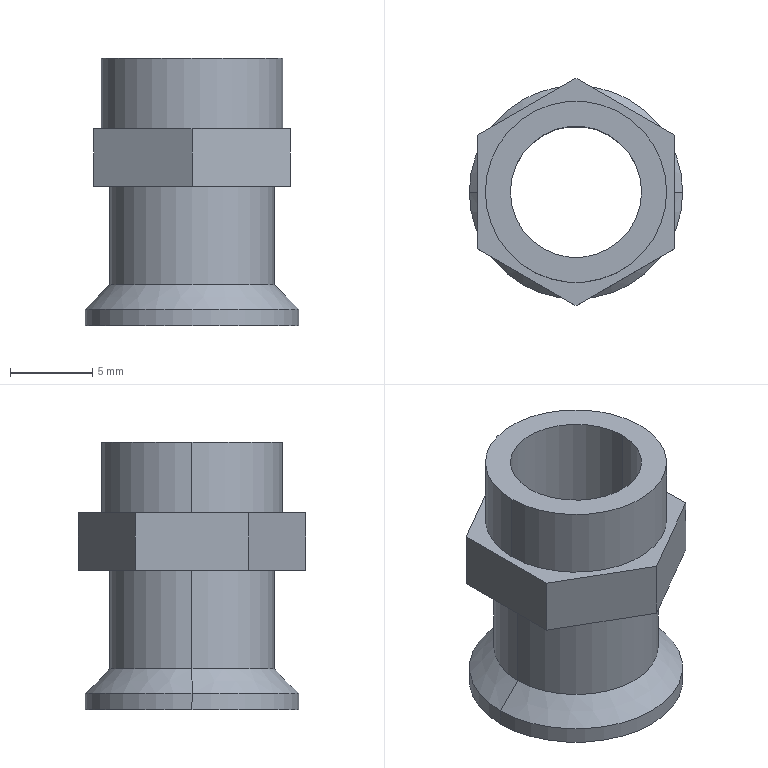Part | STEP file | Sensor nut | 1 solid | 20 faces | box 13 x 13.856 x 16.3 mm | volume 789.56 mm3 | plane 10 | cylinder 8 | cone 2 | commonest cylinder face diameters 8 x2 10 x2 11.042 x2 13 x2
STEP:
#1=CARTESIAN_POINT('',(0.,0.,0.));
#2=DIRECTION('',(0.,0.,1.));
#3=DIRECTION('',(1.,0.,0.));
#4=AXIS2_PLACEMENT_3D('',#1,#2,#3);
#5=CARTESIAN_POINT('',(-4.,0.,7.8));
#6=VERTEX_POINT('',#5);
#7=CARTESIAN_POINT('',(-4.,0.,-8.5));
#8=VERTEX_POINT('',#7);
#9=CARTESIAN_POINT('',(-4.,0.,3.5));
#10=DIRECTION('',(0.,0.,-1.));
#11=VECTOR('',#10,1.);
#12=LINE('',#9,#11);
#13=CARTESIAN_POINT('',(0.,0.,3.5));
#14=DIRECTION('',(0.,0.,-1.));
#15=DIRECTION('',(-1.,0.,0.));
#16=AXIS2_PLACEMENT_3D('',#13,#14,#15);
#17=CYLINDRICAL_SURFACE('',#16,4.);
#18=CARTESIAN_POINT('',(6.283,0.));
#19=DIRECTION('',(0.,1.));
#20=VECTOR('',#19,1.);
#21=LINE('',#18,#20);
#22=(GEOMETRIC_REPRESENTATION_CONTEXT(2)PARAMETRIC_REPRESENTATION_CONTEXT()REPRESENTATION_CONTEXT('',''));
#23=DEFINITIONAL_REPRESENTATION('',(#21),#22);
#24=PCURVE('',#17,#23);
#25=CARTESIAN_POINT('',(0.,0.,3.5));
#26=DIRECTION('',(0.,0.,-1.));
#27=DIRECTION('',(-1.,0.,0.));
#28=AXIS2_PLACEMENT_3D('',#25,#26,#27);
#29=CYLINDRICAL_SURFACE('',#28,4.);
#30=CARTESIAN_POINT('',(0.,0.));
#31=DIRECTION('',(0.,1.));
#32=VECTOR('',#31,1.);
#33=LINE('',#30,#32);
#34=(GEOMETRIC_REPRESENTATION_CONTEXT(2)PARAMETRIC_REPRESENTATION_CONTEXT()REPRESENTATION_CONTEXT('',''));
#35=DEFINITIONAL_REPRESENTATION('',(#33),#34);
#36=PCURVE('',#29,#35);
#37=SURFACE_CURVE('',#12,(#24,#36),.PCURVE_S1.);
#38=EDGE_CURVE('',#6,#8,#37,.T.);
#39=ORIENTED_EDGE('',*,*,#38,.T.);
#40=CARTESIAN_POINT('',(4.,0.,-8.5));
#41=VERTEX_POINT('',#40);
#42=CARTESIAN_POINT('',(0.,0.,-8.5));
#43=DIRECTION('',(0.,0.,1.));
#44=DIRECTION('',(-1.,0.,0.));
#45=AXIS2_PLACEMENT_3D('',#42,#43,#44);
#46=CIRCLE('',#45,4.);
#47=CARTESIAN_POINT('',(6.283,12.));
#48=DIRECTION('',(-1.,0.));
#49=VECTOR('',#48,1.);
#50=LINE('',#47,#49);
#51=(GEOMETRIC_REPRESENTATION_CONTEXT(2)PARAMETRIC_REPRESENTATION_CONTEXT()REPRESENTATION_CONTEXT('',''));
#52=DEFINITIONAL_REPRESENTATION('',(#50),#51);
#53=PCURVE('',#17,#52);
#54=CARTESIAN_POINT('',(6.5,0.,-8.5));
#55=DIRECTION('',(0.,0.,-1.));
#56=DIRECTION('',(-1.,0.,0.));
#57=AXIS2_PLACEMENT_3D('',#54,#55,#56);
#58=PLANE('',#57);
#59=CARTESIAN_POINT('',(10.5,0.));
#60=CARTESIAN_POINT('',(10.5,-6.928));
#61=CARTESIAN_POINT('',(4.5,-3.464));
#62=CARTESIAN_POINT('',(-1.5,0.));
#63=CARTESIAN_POINT('',(4.5,3.464));
#64=CARTESIAN_POINT('',(10.5,6.928));
#65=CARTESIAN_POINT('',(10.5,0.));
#66=(BOUNDED_CURVE()B_SPLINE_CURVE(2,(#59,#60,#61,#62,#63,#64,#65),.UNSPECIFIED.,.T.,.F.)B_SPLINE_CURVE_WITH_KNOTS((1,2,2,2,2,1),(-2.094,0.,2.094,4.189,6.283,8.378),.UNSPECIFIED.)CURVE()GEOMETRIC_REPRESENTATION_ITEM()RATIONAL_B_SPLINE_CURVE((1.,0.5,1.,0.5,1.,0.5,1.))REPRESENTATION_ITEM(''));
#67=(GEOMETRIC_REPRESENTATION_CONTEXT(2)PARAMETRIC_REPRESENTATION_CONTEXT()REPRESENTATION_CONTEXT('',''));
#68=DEFINITIONAL_REPRESENTATION('',(#66),#67);
#69=PCURVE('',#58,#68);
#70=SURFACE_CURVE('',#46,(#53,#69),.PCURVE_S1.);
#71=EDGE_CURVE('',#8,#41,#70,.T.);
#72=ORIENTED_EDGE('',*,*,#71,.T.);
#73=CARTESIAN_POINT('',(4.,0.,7.8));
#74=VERTEX_POINT('',#73);
#75=CARTESIAN_POINT('',(4.,0.,3.5));
#76=DIRECTION('',(0.,0.,-1.));
#77=VECTOR('',#76,1.);
#78=LINE('',#75,#77);
#79=CARTESIAN_POINT('',(3.142,0.));
#80=DIRECTION('',(0.,1.));
#81=VECTOR('',#80,1.);
#82=LINE('',#79,#81);
#83=(GEOMETRIC_REPRESENTATION_CONTEXT(2)PARAMETRIC_REPRESENTATION_CONTEXT()REPRESENTATION_CONTEXT('',''));
#84=DEFINITIONAL_REPRESENTATION('',(#82),#83);
#85=PCURVE('',#17,#84);
#86=CARTESIAN_POINT('',(3.142,0.));
#87=DIRECTION('',(0.,1.));
#88=VECTOR('',#87,1.);
#89=LINE('',#86,#88);
#90=(GEOMETRIC_REPRESENTATION_CONTEXT(2)PARAMETRIC_REPRESENTATION_CONTEXT()REPRESENTATION_CONTEXT('',''));
#91=DEFINITIONAL_REPRESENTATION('',(#89),#90);
#92=PCURVE('',#29,#91);
#93=SURFACE_CURVE('',#78,(#85,#92),.PCURVE_S1.);
#94=EDGE_CURVE('',#74,#41,#93,.T.);
#95=ORIENTED_EDGE('',*,*,#94,.F.);
#96=CARTESIAN_POINT('',(0.,0.,7.8));
#97=DIRECTION('',(0.,0.,-1.));
#98=DIRECTION('',(-1.,0.,0.));
#99=AXIS2_PLACEMENT_3D('',#96,#97,#98);
#100=CIRCLE('',#99,4.);
#101=CARTESIAN_POINT('',(0.,-4.3));
#102=DIRECTION('',(1.,0.));
#103=VECTOR('',#102,1.);
#104=LINE('',#101,#103);
#105=(GEOMETRIC_REPRESENTATION_CONTEXT(2)PARAMETRIC_REPRESENTATION_CONTEXT()REPRESENTATION_CONTEXT('',''));
#106=DEFINITIONAL_REPRESENTATION('',(#104),#105);
#107=PCURVE('',#17,#106);
#108=CARTESIAN_POINT('',(4.,0.,7.8));
#109=DIRECTION('',(0.,0.,1.));
#110=DIRECTION('',(1.,0.,0.));
#111=AXIS2_PLACEMENT_3D('',#108,#109,#110);
#112=PLANE('',#111);
#113=CARTESIAN_POINT('',(-8.,0.));
#114=CARTESIAN_POINT('',(-8.,6.928));
#115=CARTESIAN_POINT('',(-2.,3.464));
#116=CARTESIAN_POINT('',(4.,0.));
#117=CARTESIAN_POINT('',(-2.,-3.464));
#118=CARTESIAN_POINT('',(-8.,-6.928));
#119=CARTESIAN_POINT('',(-8.,0.));
#120=(BOUNDED_CURVE()B_SPLINE_CURVE(2,(#113,#114,#115,#116,#117,#118,#119),.UNSPECIFIED.,.T.,.F.)B_SPLINE_CURVE_WITH_KNOTS((1,2,2,2,2,1),(-2.094,0.,2.094,4.189,6.283,8.378),.UNSPECIFIED.)CURVE()GEOMETRIC_REPRESENTATION_ITEM()RATIONAL_B_SPLINE_CURVE((1.,0.5,1.,0.5,1.,0.5,1.))REPRESENTATION_ITEM(''));
#121=(GEOMETRIC_REPRESENTATION_CONTEXT(2)PARAMETRIC_REPRESENTATION_CONTEXT()REPRESENTATION_CONTEXT('',''));
#122=DEFINITIONAL_REPRESENTATION('',(#120),#121);
#123=PCURVE('',#112,#122);
#124=SURFACE_CURVE('',#100,(#107,#123),.PCURVE_S1.);
#125=EDGE_CURVE('',#74,#6,#124,.T.);
#126=ORIENTED_EDGE('',*,*,#125,.T.);
#127=EDGE_LOOP('',(#39,#72,#95,#126));
#128=FACE_BOUND('',#127,.F.);
#129=ADVANCED_FACE('',(#128),#17,.F.);
#130=CARTESIAN_POINT('',(5.521,0.,3.5));
#131=VERTEX_POINT('',#130);
#132=CARTESIAN_POINT('',(-5.521,0.,3.5));
#133=VERTEX_POINT('',#132);
#134=CARTESIAN_POINT('',(0.,0.,3.5));
#135=DIRECTION('',(0.,0.,1.));
#136=DIRECTION('',(1.,0.,0.));
#137=AXIS2_PLACEMENT_3D('',#134,#135,#136);
#138=CIRCLE('',#137,5.521);
#139=CARTESIAN_POINT('',(0.,0.,0.));
#140=DIRECTION('',(0.,0.,1.));
#141=DIRECTION('',(1.,0.,0.));
#142=AXIS2_PLACEMENT_3D('',#139,#140,#141);
#143=CYLINDRICAL_SURFACE('',#142,5.521);
#144=CARTESIAN_POINT('',(0.,3.5));
#145=DIRECTION('',(1.,0.));
#146=VECTOR('',#145,1.);
#147=LINE('',#144,#146);
#148=(GEOMETRIC_REPRESENTATION_CONTEXT(2)PARAMETRIC_REPRESENTATION_CONTEXT()REPRESENTATION_CONTEXT('',''));
#149=DEFINITIONAL_REPRESENTATION('',(#147),#148);
#150=PCURVE('',#143,#149);
#151=CARTESIAN_POINT('',(0.,6.928,3.5));
#152=DIRECTION('',(0.,0.,1.));
#153=DIRECTION('',(1.,0.,0.));
#154=AXIS2_PLACEMENT_3D('',#151,#152,#153);
#155=PLANE('',#154);
#156=CARTESIAN_POINT('',(0.,-6.928));
#157=DIRECTION('',(1.,0.));
#158=AXIS2_PLACEMENT_2D('',#156,#157);
#159=CIRCLE('',#158,5.521);
#160=(GEOMETRIC_REPRESENTATION_CONTEXT(2)PARAMETRIC_REPRESENTATION_CONTEXT()REPRESENTATION_CONTEXT('',''));
#161=DEFINITIONAL_REPRESENTATION('',(#159),#160);
#162=PCURVE('',#155,#161);
#163=SURFACE_CURVE('',#138,(#150,#162),.PCURVE_S1.);
#164=EDGE_CURVE('',#131,#133,#163,.T.);
#165=ORIENTED_EDGE('',*,*,#164,.T.);
#166=CARTESIAN_POINT('',(-5.521,0.,7.8));
#167=VERTEX_POINT('',#166);
#168=CARTESIAN_POINT('',(-5.521,0.,0.));
#169=DIRECTION('',(0.,0.,1.));
#170=VECTOR('',#169,1.);
#171=LINE('',#168,#170);
#172=CARTESIAN_POINT('',(3.142,0.));
#173=DIRECTION('',(0.,1.));
#174=VECTOR('',#173,1.);
#175=LINE('',#172,#174);
#176=(GEOMETRIC_REPRESENTATION_CONTEXT(2)PARAMETRIC_REPRESENTATION_CONTEXT()REPRESENTATION_CONTEXT('',''));
#177=DEFINITIONAL_REPRESENTATION('',(#175),#176);
#178=PCURVE('',#143,#177);
#179=CARTESIAN_POINT('',(0.,0.,0.));
#180=DIRECTION('',(0.,0.,1.));
#181=DIRECTION('',(1.,0.,0.));
#182=AXIS2_PLACEMENT_3D('',#179,#180,#181);
#183=CYLINDRICAL_SURFACE('',#182,5.521);
#184=CARTESIAN_POINT('',(3.142,0.));
#185=DIRECTION('',(0.,1.));
#186=VECTOR('',#185,1.);
#187=LINE('',#184,#186);
#188=(GEOMETRIC_REPRESENTATION_CONTEXT(2)PARAMETRIC_REPRESENTATION_CONTEXT()REPRESENTATION_CONTEXT('',''));
#189=DEFINITIONAL_REPRESENTATION('',(#187),#188);
#190=PCURVE('',#183,#189);
#191=SURFACE_CURVE('',#171,(#178,#190),.PCURVE_S1.);
#192=EDGE_CURVE('',#133,#167,#191,.T.);
#193=ORIENTED_EDGE('',*,*,#192,.T.);
#194=CARTESIAN_POINT('',(5.521,0.,7.8));
#195=VERTEX_POINT('',#194);
#196=CARTESIAN_POINT('',(0.,0.,7.8));
#197=DIRECTION('',(0.,0.,1.));
#198=DIRECTION('',(1.,0.,0.));
#199=AXIS2_PLACEMENT_3D('',#196,#197,#198);
#200=CIRCLE('',#199,5.521);
#201=CARTESIAN_POINT('',(0.,7.8));
#202=DIRECTION('',(1.,0.));
#203=VECTOR('',#202,1.);
#204=LINE('',#201,#203);
#205=(GEOMETRIC_REPRESENTATION_CONTEXT(2)PARAMETRIC_REPRESENTATION_CONTEXT()REPRESENTATION_CONTEXT('',''));
#206=DEFINITIONAL_REPRESENTATION('',(#204),#205);
#207=PCURVE('',#143,#206);
#208=CARTESIAN_POINT('',(-4.,0.));
#209=DIRECTION('',(1.,0.));
#210=AXIS2_PLACEMENT_2D('',#208,#209);
#211=CIRCLE('',#210,5.521);
#212=(GEOMETRIC_REPRESENTATION_CONTEXT(2)PARAMETRIC_REPRESENTATION_CONTEXT()REPRESENTATION_CONTEXT('',''));
#213=DEFINITIONAL_REPRESENTATION('',(#211),#212);
#214=PCURVE('',#112,#213);
#215=SURFACE_CURVE('',#200,(#207,#214),.PCURVE_S1.);
#216=EDGE_CURVE('',#195,#167,#215,.T.);
#217=ORIENTED_EDGE('',*,*,#216,.F.);
#218=CARTESIAN_POINT('',(5.521,0.,0.));
#219=DIRECTION('',(0.,0.,1.));
#220=VECTOR('',#219,1.);
#221=LINE('',#218,#220);
#222=CARTESIAN_POINT('',(0.,0.));
#223=DIRECTION('',(0.,1.));
#224=VECTOR('',#223,1.);
#225=LINE('',#222,#224);
#226=(GEOMETRIC_REPRESENTATION_CONTEXT(2)PARAMETRIC_REPRESENTATION_CONTEXT()REPRESENTATION_CONTEXT('',''));
#227=DEFINITIONAL_REPRESENTATION('',(#225),#226);
#228=PCURVE('',#143,#227);
#229=CARTESIAN_POINT('',(6.283,0.));
#230=DIRECTION('',(0.,1.));
#231=VECTOR('',#230,1.);
#232=LINE('',#229,#231);
#233=(GEOMETRIC_REPRESENTATION_CONTEXT(2)PARAMETRIC_REPRESENTATION_CONTEXT()REPRESENTATION_CONTEXT('',''));
#234=DEFINITIONAL_REPRESENTATION('',(#232),#233);
#235=PCURVE('',#183,#234);
#236=SURFACE_CURVE('',#221,(#228,#235),.PCURVE_S1.);
#237=EDGE_CURVE('',#131,#195,#236,.T.);
#238=ORIENTED_EDGE('',*,*,#237,.F.);
#239=EDGE_LOOP('',(#165,#193,#217,#238));
#240=FACE_BOUND('',#239,.T.);
#241=ADVANCED_FACE('',(#240),#143,.T.);
#242=CARTESIAN_POINT('',(-6.5,0.,-8.5));
#243=VERTEX_POINT('',#242);
#244=CARTESIAN_POINT('',(6.5,0.,-8.5));
#245=VERTEX_POINT('',#244);
#246=CARTESIAN_POINT('',(0.,0.,-8.5));
#247=DIRECTION('',(0.,0.,-1.));
#248=DIRECTION('',(1.,0.,0.));
#249=AXIS2_PLACEMENT_3D('',#246,#247,#248);
#250=CIRCLE('',#249,6.5);
#251=CARTESIAN_POINT('',(0.,0.,0.));
#252=DIRECTION('',(0.,0.,1.));
#253=DIRECTION('',(1.,0.,0.));
#254=AXIS2_PLACEMENT_3D('',#251,#252,#253);
#255=CYLINDRICAL_SURFACE('',#254,6.5);
#256=CARTESIAN_POINT('',(6.283,-8.5));
#257=DIRECTION('',(-1.,0.));
#258=VECTOR('',#257,1.);
#259=LINE('',#256,#258);
#260=(GEOMETRIC_REPRESENTATION_CONTEXT(2)PARAMETRIC_REPRESENTATION_CONTEXT()REPRESENTATION_CONTEXT('',''));
#261=DEFINITIONAL_REPRESENTATION('',(#259),#260);
#262=PCURVE('',#255,#261);
#263=CARTESIAN_POINT('',(6.5,0.));
#264=DIRECTION('',(-1.,0.));
#265=AXIS2_PLACEMENT_2D('',#263,#264);
#266=CIRCLE('',#265,6.5);
#267=(GEOMETRIC_REPRESENTATION_CONTEXT(2)PARAMETRIC_REPRESENTATION_CONTEXT()REPRESENTATION_CONTEXT('',''));
#268=DEFINITIONAL_REPRESENTATION('',(#266),#267);
#269=PCURVE('',#58,#268);
#270=SURFACE_CURVE('',#250,(#262,#269),.PCURVE_S1.);
#271=EDGE_CURVE('',#243,#245,#270,.T.);
#272=ORIENTED_EDGE('',*,*,#271,.F.);
#273=CARTESIAN_POINT('',(-6.5,0.,-7.5));
#274=VERTEX_POINT('',#273);
#275=CARTESIAN_POINT('',(-6.5,0.,0.));
#276=DIRECTION('',(0.,0.,1.));
#277=VECTOR('',#276,1.);
#278=LINE('',#275,#277);
#279=CARTESIAN_POINT('',(3.142,0.));
#280=DIRECTION('',(0.,1.));
#281=VECTOR('',#280,1.);
#282=LINE('',#279,#281);
#283=(GEOMETRIC_REPRESENTATION_CONTEXT(2)PARAMETRIC_REPRESENTATION_CONTEXT()REPRESENTATION_CONTEXT('',''));
#284=DEFINITIONAL_REPRESENTATION('',(#282),#283);
#285=PCURVE('',#255,#284);
#286=CARTESIAN_POINT('',(0.,0.,0.));
#287=DIRECTION('',(0.,0.,1.));
#288=DIRECTION('',(1.,0.,0.));
#289=AXIS2_PLACEMENT_3D('',#286,#287,#288);
#290=CYLINDRICAL_SURFACE('',#289,6.5);
#291=CARTESIAN_POINT('',(3.142,0.));
#292=DIRECTION('',(0.,1.));
#293=VECTOR('',#292,1.);
#294=LINE('',#291,#293);
#295=(GEOMETRIC_REPRESENTATION_CONTEXT(2)PARAMETRIC_REPRESENTATION_CONTEXT()REPRESENTATION_CONTEXT('',''));
#296=DEFINITIONAL_REPRESENTATION('',(#294),#295);
#297=PCURVE('',#290,#296);
#298=SURFACE_CURVE('',#278,(#285,#297),.PCURVE_S1.);
#299=EDGE_CURVE('',#243,#274,#298,.T.);
#300=ORIENTED_EDGE('',*,*,#299,.T.);
#301=CARTESIAN_POINT('',(6.5,0.,-7.5));
#302=VERTEX_POINT('',#301);
#303=CARTESIAN_POINT('',(0.,0.,-7.5));
#304=DIRECTION('',(0.,0.,-1.));
#305=DIRECTION('',(1.,0.,0.));
#306=AXIS2_PLACEMENT_3D('',#303,#304,#305);
#307=CIRCLE('',#306,6.5);
#308=CARTESIAN_POINT('',(6.283,-7.5));
#309=DIRECTION('',(-1.,0.));
#310=VECTOR('',#309,1.);
#311=LINE('',#308,#310);
#312=(GEOMETRIC_REPRESENTATION_CONTEXT(2)PARAMETRIC_REPRESENTATION_CONTEXT()REPRESENTATION_CONTEXT('',''));
#313=DEFINITIONAL_REPRESENTATION('',(#311),#312);
#314=PCURVE('',#255,#313);
#315=CARTESIAN_POINT('',(0.,0.,-7.5));
#316=DIRECTION('',(0.,0.,-1.));
#317=DIRECTION('',(-1.,0.,0.));
#318=AXIS2_PLACEMENT_3D('',#315,#316,#317);
#319=CONICAL_SURFACE('',#318,6.5,0.7854);
#320=CARTESIAN_POINT('',(-3.142,0.));
#321=DIRECTION('',(1.,0.));
#322=VECTOR('',#321,1.);
#323=LINE('',#320,#322);
#324=(GEOMETRIC_REPRESENTATION_CONTEXT(2)PARAMETRIC_REPRESENTATION_CONTEXT()REPRESENTATION_CONTEXT('',''));
#325=DEFINITIONAL_REPRESENTATION('',(#323),#324);
#326=PCURVE('',#319,#325);
#327=SURFACE_CURVE('',#307,(#314,#326),.PCURVE_S1.);
#328=EDGE_CURVE('',#274,#302,#327,.T.);
#329=ORIENTED_EDGE('',*,*,#328,.T.);
#330=CARTESIAN_POINT('',(6.5,0.,0.));
#331=DIRECTION('',(0.,0.,1.));
#332=VECTOR('',#331,1.);
#333=LINE('',#330,#332);
#334=CARTESIAN_POINT('',(0.,0.));
#335=DIRECTION('',(0.,1.));
#336=VECTOR('',#335,1.);
#337=LINE('',#334,#336);
#338=(GEOMETRIC_REPRESENTATION_CONTEXT(2)PARAMETRIC_REPRESENTATION_CONTEXT()REPRESENTATION_CONTEXT('',''));
#339=DEFINITIONAL_REPRESENTATION('',(#337),#338);
#340=PCURVE('',#255,#339);
#341=CARTESIAN_POINT('',(6.283,0.));
#342=DIRECTION('',(0.,1.));
#343=VECTOR('',#342,1.);
#344=LINE('',#341,#343);
#345=(GEOMETRIC_REPRESENTATION_CONTEXT(2)PARAMETRIC_REPRESENTATION_CONTEXT()REPRESENTATION_CONTEXT('',''));
#346=DEFINITIONAL_REPRESENTATION('',(#344),#345);
#347=PCURVE('',#290,#346);
#348=SURFACE_CURVE('',#333,(#340,#347),.PCURVE_S1.);
#349=EDGE_CURVE('',#245,#302,#348,.T.);
#350=ORIENTED_EDGE('',*,*,#349,.F.);
#351=EDGE_LOOP('',(#272,#300,#329,#350));
#352=FACE_BOUND('',#351,.T.);
#353=ADVANCED_FACE('',(#352),#255,.T.);
#354=CARTESIAN_POINT('',(-5.,0.,-6.));
#355=VERTEX_POINT('',#354);
#356=CARTESIAN_POINT('',(5.,0.,-6.));
#357=VERTEX_POINT('',#356);
#358=CARTESIAN_POINT('',(0.,0.,-6.));
#359=DIRECTION('',(0.,0.,-1.));
#360=DIRECTION('',(-1.,0.,0.));
#361=AXIS2_PLACEMENT_3D('',#358,#359,#360);
#362=CIRCLE('',#361,5.);
#363=CARTESIAN_POINT('',(0.,-1.5));
#364=DIRECTION('',(1.,0.));
#365=VECTOR('',#364,1.);
#366=LINE('',#363,#365);
#367=(GEOMETRIC_REPRESENTATION_CONTEXT(2)PARAMETRIC_REPRESENTATION_CONTEXT()REPRESENTATION_CONTEXT('',''));
#368=DEFINITIONAL_REPRESENTATION('',(#366),#367);
#369=PCURVE('',#319,#368);
#370=CARTESIAN_POINT('',(0.,0.,0.));
#371=DIRECTION('',(0.,0.,1.));
#372=DIRECTION('',(1.,0.,0.));
#373=AXIS2_PLACEMENT_3D('',#370,#371,#372);
#374=CYLINDRICAL_SURFACE('',#373,5.);
#375=CARTESIAN_POINT('',(3.142,-6.));
#376=DIRECTION('',(-1.,0.));
#377=VECTOR('',#376,1.);
#378=LINE('',#375,#377);
#379=(GEOMETRIC_REPRESENTATION_CONTEXT(2)PARAMETRIC_REPRESENTATION_CONTEXT()REPRESENTATION_CONTEXT('',''));
#380=DEFINITIONAL_REPRESENTATION('',(#378),#379);
#381=PCURVE('',#374,#380);
#382=SURFACE_CURVE('',#362,(#369,#381),.PCURVE_S1.);
#383=EDGE_CURVE('',#355,#357,#382,.T.);
#384=ORIENTED_EDGE('',*,*,#383,.T.);
#385=CARTESIAN_POINT('',(6.5,0.,-7.5));
#386=DIRECTION('',(0.7071,0.,-0.7071));
#387=VECTOR('',#386,1.);
#388=LINE('',#385,#387);
#389=CARTESIAN_POINT('',(3.142,0.));
#390=DIRECTION('',(0.,1.));
#391=VECTOR('',#390,1.);
#392=LINE('',#389,#391);
#393=(GEOMETRIC_REPRESENTATION_CONTEXT(2)PARAMETRIC_REPRESENTATION_CONTEXT()REPRESENTATION_CONTEXT('',''));
#394=DEFINITIONAL_REPRESENTATION('',(#392),#393);
#395=PCURVE('',#319,#394);
#396=CARTESIAN_POINT('',(0.,0.,-7.5));
#397=DIRECTION('',(0.,0.,-1.));
#398=DIRECTION('',(-1.,0.,0.));
#399=AXIS2_PLACEMENT_3D('',#396,#397,#398);
#400=CONICAL_SURFACE('',#399,6.5,0.7854);
#401=CARTESIAN_POINT('',(3.142,0.));
#402=DIRECTION('',(0.,1.));
#403=VECTOR('',#402,1.);
#404=LINE('',#401,#403);
#405=(GEOMETRIC_REPRESENTATION_CONTEXT(2)PARAMETRIC_REPRESENTATION_CONTEXT()REPRESENTATION_CONTEXT('',''));
#406=DEFINITIONAL_REPRESENTATION('',(#404),#405);
#407=PCURVE('',#400,#406);
#408=SURFACE_CURVE('',#388,(#395,#407),.PCURVE_S1.);
#409=EDGE_CURVE('',#357,#302,#408,.T.);
#410=ORIENTED_EDGE('',*,*,#409,.T.);
#411=ORIENTED_EDGE('',*,*,#328,.F.);
#412=CARTESIAN_POINT('',(-6.5,0.,-7.5));
#413=DIRECTION('',(-0.7071,0.,-0.7071));
#414=VECTOR('',#413,1.);
#415=LINE('',#412,#414);
#416=CARTESIAN_POINT('',(0.,0.));
#417=DIRECTION('',(0.,1.));
#418=VECTOR('',#417,1.);
#419=LINE('',#416,#418);
#420=(GEOMETRIC_REPRESENTATION_CONTEXT(2)PARAMETRIC_REPRESENTATION_CONTEXT()REPRESENTATION_CONTEXT('',''));
#421=DEFINITIONAL_REPRESENTATION('',(#419),#420);
#422=PCURVE('',#319,#421);
#423=CARTESIAN_POINT('',(6.283,0.));
#424=DIRECTION('',(0.,1.));
#425=VECTOR('',#424,1.);
#426=LINE('',#423,#425);
#427=(GEOMETRIC_REPRESENTATION_CONTEXT(2)PARAMETRIC_REPRESENTATION_CONTEXT()REPRESENTATION_CONTEXT('',''));
#428=DEFINITIONAL_REPRESENTATION('',(#426),#427);
#429=PCURVE('',#400,#428);
#430=SURFACE_CURVE('',#415,(#422,#429),.PCURVE_S1.);
#431=EDGE_CURVE('',#355,#274,#430,.T.);
#432=ORIENTED_EDGE('',*,*,#431,.F.);
#433=EDGE_LOOP('',(#384,#410,#411,#432));
#434=FACE_BOUND('',#433,.T.);
#435=ADVANCED_FACE('',(#434),#319,.T.);
#436=ORIENTED_EDGE('',*,*,#383,.F.);
#437=CARTESIAN_POINT('',(-5.,0.,0.));
#438=VERTEX_POINT('',#437);
#439=CARTESIAN_POINT('',(-5.,0.,0.));
#440=DIRECTION('',(0.,0.,1.));
#441=VECTOR('',#440,1.);
#442=LINE('',#439,#441);
#443=CARTESIAN_POINT('',(3.142,0.));
#444=DIRECTION('',(0.,1.));
#445=VECTOR('',#444,1.);
#446=LINE('',#443,#445);
#447=(GEOMETRIC_REPRESENTATION_CONTEXT(2)PARAMETRIC_REPRESENTATION_CONTEXT()REPRESENTATION_CONTEXT('',''));
#448=DEFINITIONAL_REPRESENTATION('',(#446),#447);
#449=PCURVE('',#374,#448);
#450=CARTESIAN_POINT('',(0.,0.,0.));
#451=DIRECTION('',(0.,0.,1.));
#452=DIRECTION('',(1.,0.,0.));
#453=AXIS2_PLACEMENT_3D('',#450,#451,#452);
#454=CYLINDRICAL_SURFACE('',#453,5.);
#455=CARTESIAN_POINT('',(3.142,0.));
#456=DIRECTION('',(0.,1.));
#457=VECTOR('',#456,1.);
#458=LINE('',#455,#457);
#459=(GEOMETRIC_REPRESENTATION_CONTEXT(2)PARAMETRIC_REPRESENTATION_CONTEXT()REPRESENTATION_CONTEXT('',''));
#460=DEFINITIONAL_REPRESENTATION('',(#458),#459);
#461=PCURVE('',#454,#460);
#462=SURFACE_CURVE('',#442,(#449,#461),.PCURVE_S1.);
#463=EDGE_CURVE('',#355,#438,#462,.T.);
#464=ORIENTED_EDGE('',*,*,#463,.T.);
#465=CARTESIAN_POINT('',(5.,0.,0.));
#466=VERTEX_POINT('',#465);
#467=CARTESIAN_POINT('',(0.,0.,0.));
#468=DIRECTION('',(0.,0.,-1.));
#469=DIRECTION('',(1.,0.,0.));
#470=AXIS2_PLACEMENT_3D('',#467,#468,#469);
#471=CIRCLE('',#470,5.);
#472=CARTESIAN_POINT('',(6.283,0.));
#473=DIRECTION('',(-1.,0.));
#474=VECTOR('',#473,1.);
#475=LINE('',#472,#474);
#476=(GEOMETRIC_REPRESENTATION_CONTEXT(2)PARAMETRIC_REPRESENTATION_CONTEXT()REPRESENTATION_CONTEXT('',''));
#477=DEFINITIONAL_REPRESENTATION('',(#475),#476);
#478=PCURVE('',#374,#477);
#479=CARTESIAN_POINT('',(0.,6.928,0.));
#480=DIRECTION('',(0.,0.,1.));
#481=DIRECTION('',(1.,0.,0.));
#482=AXIS2_PLACEMENT_3D('',#479,#480,#481);
#483=PLANE('',#482);
#484=CARTESIAN_POINT('',(5.,-6.928));
#485=CARTESIAN_POINT('',(5.,-15.588));
#486=CARTESIAN_POINT('',(-2.5,-11.258));
#487=CARTESIAN_POINT('',(-10.,-6.928));
#488=CARTESIAN_POINT('',(-2.5,-2.598));
#489=CARTESIAN_POINT('',(5.,1.732));
#490=CARTESIAN_POINT('',(5.,-6.928));
#491=(BOUNDED_CURVE()B_SPLINE_CURVE(2,(#484,#485,#486,#487,#488,#489,#490),.UNSPECIFIED.,.T.,.F.)B_SPLINE_CURVE_WITH_KNOTS((1,2,2,2,2,1),(-2.094,0.,2.094,4.189,6.283,8.378),.UNSPECIFIED.)CURVE()GEOMETRIC_REPRESENTATION_ITEM()RATIONAL_B_SPLINE_CURVE((1.,0.5,1.,0.5,1.,0.5,1.))REPRESENTATION_ITEM(''));
#492=(GEOMETRIC_REPRESENTATION_CONTEXT(2)PARAMETRIC_REPRESENTATION_CONTEXT()REPRESENTATION_CONTEXT('',''));
#493=DEFINITIONAL_REPRESENTATION('',(#491),#492);
#494=PCURVE('',#483,#493);
#495=SURFACE_CURVE('',#471,(#478,#494),.PCURVE_S1.);
#496=EDGE_CURVE('',#438,#466,#495,.T.);
#497=ORIENTED_EDGE('',*,*,#496,.T.);
#498=CARTESIAN_POINT('',(5.,0.,0.));
#499=DIRECTION('',(0.,0.,1.));
#500=VECTOR('',#499,1.);
#501=LINE('',#498,#500);
#502=CARTESIAN_POINT('',(0.,0.));
#503=DIRECTION('',(0.,1.));
#504=VECTOR('',#503,1.);
#505=LINE('',#502,#504);
#506=(GEOMETRIC_REPRESENTATION_CONTEXT(2)PARAMETRIC_REPRESENTATION_CONTEXT()REPRESENTATION_CONTEXT('',''));
#507=DEFINITIONAL_REPRESENTATION('',(#505),#506);
#508=PCURVE('',#374,#507);
#509=CARTESIAN_POINT('',(6.283,0.));
#510=DIRECTION('',(0.,1.));
#511=VECTOR('',#510,1.);
#512=LINE('',#509,#511);
#513=(GEOMETRIC_REPRESENTATION_CONTEXT(2)PARAMETRIC_REPRESENTATION_CONTEXT()REPRESENTATION_CONTEXT('',''));
#514=DEFINITIONAL_REPRESENTATION('',(#512),#513);
#515=PCURVE('',#454,#514);
#516=SURFACE_CURVE('',#501,(#508,#515),.PCURVE_S1.);
#517=EDGE_CURVE('',#357,#466,#516,.T.);
#518=ORIENTED_EDGE('',*,*,#517,.F.);
#519=EDGE_LOOP('',(#436,#464,#497,#518));
#520=FACE_BOUND('',#519,.T.);
#521=ADVANCED_FACE('',(#520),#374,.T.);
#522=CARTESIAN_POINT('',(0.,0.,-8.5));
#523=DIRECTION('',(0.,0.,1.));
#524=DIRECTION('',(-1.,0.,0.));
#525=AXIS2_PLACEMENT_3D('',#522,#523,#524);
#526=CIRCLE('',#525,4.);
#527=CARTESIAN_POINT('',(6.283,12.));
#528=DIRECTION('',(-1.,0.));
#529=VECTOR('',#528,1.);
#530=LINE('',#527,#529);
#531=(GEOMETRIC_REPRESENTATION_CONTEXT(2)PARAMETRIC_REPRESENTATION_CONTEXT()REPRESENTATION_CONTEXT('',''));
#532=DEFINITIONAL_REPRESENTATION('',(#530),#531);
#533=PCURVE('',#29,#532);
#534=CARTESIAN_POINT('',(10.5,0.));
#535=CARTESIAN_POINT('',(10.5,-6.928));
#536=CARTESIAN_POINT('',(4.5,-3.464));
#537=CARTESIAN_POINT('',(-1.5,0.));
#538=CARTESIAN_POINT('',(4.5,3.464));
#539=CARTESIAN_POINT('',(10.5,6.928));
#540=CARTESIAN_POINT('',(10.5,0.));
#541=(BOUNDED_CURVE()B_SPLINE_CURVE(2,(#534,#535,#536,#537,#538,#539,#540),.UNSPECIFIED.,.T.,.F.)B_SPLINE_CURVE_WITH_KNOTS((1,2,2,2,2,1),(-2.094,0.,2.094,4.189,6.283,8.378),.UNSPECIFIED.)CURVE()GEOMETRIC_REPRESENTATION_ITEM()RATIONAL_B_SPLINE_CURVE((1.,0.5,1.,0.5,1.,0.5,1.))REPRESENTATION_ITEM(''));
#542=(GEOMETRIC_REPRESENTATION_CONTEXT(2)PARAMETRIC_REPRESENTATION_CONTEXT()REPRESENTATION_CONTEXT('',''));
#543=DEFINITIONAL_REPRESENTATION('',(#541),#542);
#544=PCURVE('',#58,#543);
#545=SURFACE_CURVE('',#526,(#533,#544),.PCURVE_S1.);
#546=EDGE_CURVE('',#41,#8,#545,.T.);
#547=ORIENTED_EDGE('',*,*,#546,.T.);
#548=ORIENTED_EDGE('',*,*,#38,.F.);
#549=CARTESIAN_POINT('',(0.,0.,7.8));
#550=DIRECTION('',(0.,0.,-1.));
#551=DIRECTION('',(-1.,0.,0.));
#552=AXIS2_PLACEMENT_3D('',#549,#550,#551);
#553=CIRCLE('',#552,4.);
#554=CARTESIAN_POINT('',(0.,-4.3));
#555=DIRECTION('',(1.,0.));
#556=VECTOR('',#555,1.);
#557=LINE('',#554,#556);
#558=(GEOMETRIC_REPRESENTATION_CONTEXT(2)PARAMETRIC_REPRESENTATION_CONTEXT()REPRESENTATION_CONTEXT('',''));
#559=DEFINITIONAL_REPRESENTATION('',(#557),#558);
#560=PCURVE('',#29,#559);
#561=CARTESIAN_POINT('',(-8.,0.));
#562=CARTESIAN_POINT('',(-8.,6.928));
#563=CARTESIAN_POINT('',(-2.,3.464));
#564=CARTESIAN_POINT('',(4.,0.));
#565=CARTESIAN_POINT('',(-2.,-3.464));
#566=CARTESIAN_POINT('',(-8.,-6.928));
#567=CARTESIAN_POINT('',(-8.,0.));
#568=(BOUNDED_CURVE()B_SPLINE_CURVE(2,(#561,#562,#563,#564,#565,#566,#567),.UNSPECIFIED.,.T.,.F.)B_SPLINE_CURVE_WITH_KNOTS((1,2,2,2,2,1),(-2.094,0.,2.094,4.189,6.283,8.378),.UNSPECIFIED.)CURVE()GEOMETRIC_REPRESENTATION_ITEM()RATIONAL_B_SPLINE_CURVE((1.,0.5,1.,0.5,1.,0.5,1.))REPRESENTATION_ITEM(''));
#569=(GEOMETRIC_REPRESENTATION_CONTEXT(2)PARAMETRIC_REPRESENTATION_CONTEXT()REPRESENTATION_CONTEXT('',''));
#570=DEFINITIONAL_REPRESENTATION('',(#568),#569);
#571=PCURVE('',#112,#570);
#572=SURFACE_CURVE('',#553,(#560,#571),.PCURVE_S1.);
#573=EDGE_CURVE('',#6,#74,#572,.T.);
#574=ORIENTED_EDGE('',*,*,#573,.T.);
#575=ORIENTED_EDGE('',*,*,#94,.T.);
#576=EDGE_LOOP('',(#547,#548,#574,#575));
#577=FACE_BOUND('',#576,.F.);
#578=ADVANCED_FACE('',(#577),#29,.F.);
#579=ORIENTED_EDGE('',*,*,#573,.T.);
#580=ORIENTED_EDGE('',*,*,#125,.T.);
#581=EDGE_LOOP('',(#579,#580));
#582=FACE_BOUND('',#581,.T.);
#583=ORIENTED_EDGE('',*,*,#216,.T.);
#584=CARTESIAN_POINT('',(0.,0.,7.8));
#585=DIRECTION('',(0.,0.,1.));
#586=DIRECTION('',(1.,0.,0.));
#587=AXIS2_PLACEMENT_3D('',#584,#585,#586);
#588=CIRCLE('',#587,5.521);
#589=CARTESIAN_POINT('',(-4.,0.));
#590=DIRECTION('',(1.,0.));
#591=AXIS2_PLACEMENT_2D('',#589,#590);
#592=CIRCLE('',#591,5.521);
#593=(GEOMETRIC_REPRESENTATION_CONTEXT(2)PARAMETRIC_REPRESENTATION_CONTEXT()REPRESENTATION_CONTEXT('',''));
#594=DEFINITIONAL_REPRESENTATION('',(#592),#593);
#595=PCURVE('',#112,#594);
#596=CARTESIAN_POINT('',(0.,7.8));
#597=DIRECTION('',(1.,0.));
#598=VECTOR('',#597,1.);
#599=LINE('',#596,#598);
#600=(GEOMETRIC_REPRESENTATION_CONTEXT(2)PARAMETRIC_REPRESENTATION_CONTEXT()REPRESENTATION_CONTEXT('',''));
#601=DEFINITIONAL_REPRESENTATION('',(#599),#600);
#602=PCURVE('',#183,#601);
#603=SURFACE_CURVE('',#588,(#595,#602),.PCURVE_S1.);
#604=EDGE_CURVE('',#167,#195,#603,.T.);
#605=ORIENTED_EDGE('',*,*,#604,.T.);
#606=EDGE_LOOP('',(#583,#605));
#607=FACE_BOUND('',#606,.T.);
#608=ADVANCED_FACE('',(#582,#607),#112,.T.);
#609=CARTESIAN_POINT('',(0.,0.,-8.5));
#610=DIRECTION('',(0.,0.,-1.));
#611=DIRECTION('',(1.,0.,0.));
#612=AXIS2_PLACEMENT_3D('',#609,#610,#611);
#613=CIRCLE('',#612,6.5);
#614=CARTESIAN_POINT('',(6.5,0.));
#615=DIRECTION('',(-1.,0.));
#616=AXIS2_PLACEMENT_2D('',#614,#615);
#617=CIRCLE('',#616,6.5);
#618=(GEOMETRIC_REPRESENTATION_CONTEXT(2)PARAMETRIC_REPRESENTATION_CONTEXT()REPRESENTATION_CONTEXT('',''));
#619=DEFINITIONAL_REPRESENTATION('',(#617),#618);
#620=PCURVE('',#58,#619);
#621=CARTESIAN_POINT('',(6.283,-8.5));
#622=DIRECTION('',(-1.,0.));
#623=VECTOR('',#622,1.);
#624=LINE('',#621,#623);
#625=(GEOMETRIC_REPRESENTATION_CONTEXT(2)PARAMETRIC_REPRESENTATION_CONTEXT()REPRESENTATION_CONTEXT('',''));
#626=DEFINITIONAL_REPRESENTATION('',(#624),#625);
#627=PCURVE('',#290,#626);
#628=SURFACE_CURVE('',#613,(#620,#627),.PCURVE_S1.);
#629=EDGE_CURVE('',#245,#243,#628,.T.);
#630=ORIENTED_EDGE('',*,*,#629,.T.);
#631=ORIENTED_EDGE('',*,*,#271,.T.);
#632=EDGE_LOOP('',(#630,#631));
#633=FACE_BOUND('',#632,.T.);
#634=ORIENTED_EDGE('',*,*,#71,.T.);
#635=ORIENTED_EDGE('',*,*,#546,.T.);
#636=EDGE_LOOP('',(#634,#635));
#637=FACE_BOUND('',#636,.T.);
#638=ADVANCED_FACE('',(#633,#637),#58,.T.);
#639=ORIENTED_EDGE('',*,*,#192,.F.);
#640=CARTESIAN_POINT('',(0.,0.,3.5));
#641=DIRECTION('',(0.,0.,1.));
#642=DIRECTION('',(1.,0.,0.));
#643=AXIS2_PLACEMENT_3D('',#640,#641,#642);
#644=CIRCLE('',#643,5.521);
#645=CARTESIAN_POINT('',(0.,3.5));
#646=DIRECTION('',(1.,0.));
#647=VECTOR('',#646,1.);
#648=LINE('',#645,#647);
#649=(GEOMETRIC_REPRESENTATION_CONTEXT(2)PARAMETRIC_REPRESENTATION_CONTEXT()REPRESENTATION_CONTEXT('',''));
#650=DEFINITIONAL_REPRESENTATION('',(#648),#649);
#651=PCURVE('',#183,#650);
#652=CARTESIAN_POINT('',(0.,-6.928));
#653=DIRECTION('',(1.,0.));
#654=AXIS2_PLACEMENT_2D('',#652,#653);
#655=CIRCLE('',#654,5.521);
#656=(GEOMETRIC_REPRESENTATION_CONTEXT(2)PARAMETRIC_REPRESENTATION_CONTEXT()REPRESENTATION_CONTEXT('',''));
#657=DEFINITIONAL_REPRESENTATION('',(#655),#656);
#658=PCURVE('',#155,#657);
#659=SURFACE_CURVE('',#644,(#651,#658),.PCURVE_S1.);
#660=EDGE_CURVE('',#133,#131,#659,.T.);
#661=ORIENTED_EDGE('',*,*,#660,.T.);
#662=ORIENTED_EDGE('',*,*,#237,.T.);
#663=ORIENTED_EDGE('',*,*,#604,.F.);
#664=EDGE_LOOP('',(#639,#661,#662,#663));
#665=FACE_BOUND('',#664,.T.);
#666=ADVANCED_FACE('',(#665),#183,.T.);
#667=ORIENTED_EDGE('',*,*,#299,.F.);
#668=ORIENTED_EDGE('',*,*,#629,.F.);
#669=ORIENTED_EDGE('',*,*,#349,.T.);
#670=CARTESIAN_POINT('',(0.,0.,-7.5));
#671=DIRECTION('',(0.,0.,-1.));
#672=DIRECTION('',(1.,0.,0.));
#673=AXIS2_PLACEMENT_3D('',#670,#671,#672);
#674=CIRCLE('',#673,6.5);
#675=CARTESIAN_POINT('',(6.283,-7.5));
#676=DIRECTION('',(-1.,0.));
#677=VECTOR('',#676,1.);
#678=LINE('',#675,#677);
#679=(GEOMETRIC_REPRESENTATION_CONTEXT(2)PARAMETRIC_REPRESENTATION_CONTEXT()REPRESENTATION_CONTEXT('',''));
#680=DEFINITIONAL_REPRESENTATION('',(#678),#679);
#681=PCURVE('',#290,#680);
#682=CARTESIAN_POINT('',(3.142,0.));
#683=DIRECTION('',(1.,0.));
#684=VECTOR('',#683,1.);
#685=LINE('',#682,#684);
#686=(GEOMETRIC_REPRESENTATION_CONTEXT(2)PARAMETRIC_REPRESENTATION_CONTEXT()REPRESENTATION_CONTEXT('',''));
#687=DEFINITIONAL_REPRESENTATION('',(#685),#686);
#688=PCURVE('',#400,#687);
#689=SURFACE_CURVE('',#674,(#681,#688),.PCURVE_S1.);
#690=EDGE_CURVE('',#302,#274,#689,.T.);
#691=ORIENTED_EDGE('',*,*,#690,.T.);
#692=EDGE_LOOP('',(#667,#668,#669,#691));
#693=FACE_BOUND('',#692,.T.);
#694=ADVANCED_FACE('',(#693),#290,.T.);
#695=CARTESIAN_POINT('',(0.,-6.928,3.5));
#696=VERTEX_POINT('',#695);
#697=CARTESIAN_POINT('',(6.,-3.464,3.5));
#698=VERTEX_POINT('',#697);
#699=CARTESIAN_POINT('',(0.,-6.928,3.5));
#700=DIRECTION('',(0.866,0.5,0.));
#701=VECTOR('',#700,1.);
#702=LINE('',#699,#701);
#703=CARTESIAN_POINT('',(0.,-13.856));
#704=DIRECTION('',(0.866,0.5));
#705=VECTOR('',#704,1.);
#706=LINE('',#703,#705);
#707=(GEOMETRIC_REPRESENTATION_CONTEXT(2)PARAMETRIC_REPRESENTATION_CONTEXT()REPRESENTATION_CONTEXT('',''));
#708=DEFINITIONAL_REPRESENTATION('',(#706),#707);
#709=PCURVE('',#155,#708);
#710=CARTESIAN_POINT('',(0.,-6.928,3.5));
#711=DIRECTION('',(-0.5,0.866,0.));
#712=DIRECTION('',(-0.866,-0.5,0.));
#713=AXIS2_PLACEMENT_3D('',#710,#711,#712);
#714=PLANE('',#713);
#715=CARTESIAN_POINT('',(0.,0.));
#716=DIRECTION('',(-1.,0.));
#717=VECTOR('',#716,1.);
#718=LINE('',#715,#717);
#719=(GEOMETRIC_REPRESENTATION_CONTEXT(2)PARAMETRIC_REPRESENTATION_CONTEXT()REPRESENTATION_CONTEXT('',''));
#720=DEFINITIONAL_REPRESENTATION('',(#718),#719);
#721=PCURVE('',#714,#720);
#722=SURFACE_CURVE('',#702,(#709,#721),.PCURVE_S1.);
#723=EDGE_CURVE('',#696,#698,#722,.T.);
#724=ORIENTED_EDGE('',*,*,#723,.T.);
#725=CARTESIAN_POINT('',(6.,3.464,3.5));
#726=VERTEX_POINT('',#725);
#727=CARTESIAN_POINT('',(6.,6.928,3.5));
#728=DIRECTION('',(0.,1.,0.));
#729=VECTOR('',#728,1.);
#730=LINE('',#727,#729);
#731=CARTESIAN_POINT('',(6.,0.));
#732=DIRECTION('',(0.,1.));
#733=VECTOR('',#732,1.);
#734=LINE('',#731,#733);
#735=(GEOMETRIC_REPRESENTATION_CONTEXT(2)PARAMETRIC_REPRESENTATION_CONTEXT()REPRESENTATION_CONTEXT('',''));
#736=DEFINITIONAL_REPRESENTATION('',(#734),#735);
#737=PCURVE('',#155,#736);
#738=CARTESIAN_POINT('',(6.,-3.464,3.5));
#739=DIRECTION('',(-1.,0.,0.));
#740=DIRECTION('',(0.,-1.,0.));
#741=AXIS2_PLACEMENT_3D('',#738,#739,#740);
#742=PLANE('',#741);
#743=CARTESIAN_POINT('',(-10.392,0.));
#744=DIRECTION('',(-1.,0.));
#745=VECTOR('',#744,1.);
#746=LINE('',#743,#745);
#747=(GEOMETRIC_REPRESENTATION_CONTEXT(2)PARAMETRIC_REPRESENTATION_CONTEXT()REPRESENTATION_CONTEXT('',''));
#748=DEFINITIONAL_REPRESENTATION('',(#746),#747);
#749=PCURVE('',#742,#748);
#750=SURFACE_CURVE('',#730,(#737,#749),.PCURVE_S1.);
#751=EDGE_CURVE('',#698,#726,#750,.T.);
#752=ORIENTED_EDGE('',*,*,#751,.T.);
#753=CARTESIAN_POINT('',(0.,6.928,3.5));
#754=VERTEX_POINT('',#753);
#755=CARTESIAN_POINT('',(6.,3.464,3.5));
#756=DIRECTION('',(-0.866,0.5,0.));
#757=VECTOR('',#756,1.);
#758=LINE('',#755,#757);
#759=CARTESIAN_POINT('',(6.,-3.464));
#760=DIRECTION('',(-0.866,0.5));
#761=VECTOR('',#760,1.);
#762=LINE('',#759,#761);
#763=(GEOMETRIC_REPRESENTATION_CONTEXT(2)PARAMETRIC_REPRESENTATION_CONTEXT()REPRESENTATION_CONTEXT('',''));
#764=DEFINITIONAL_REPRESENTATION('',(#762),#763);
#765=PCURVE('',#155,#764);
#766=CARTESIAN_POINT('',(6.,3.464,3.5));
#767=DIRECTION('',(-0.5,-0.866,0.));
#768=DIRECTION('',(0.866,-0.5,0.));
#769=AXIS2_PLACEMENT_3D('',#766,#767,#768);
#770=PLANE('',#769);
#771=CARTESIAN_POINT('',(0.,0.));
#772=DIRECTION('',(-1.,0.));
#773=VECTOR('',#772,1.);
#774=LINE('',#771,#773);
#775=(GEOMETRIC_REPRESENTATION_CONTEXT(2)PARAMETRIC_REPRESENTATION_CONTEXT()REPRESENTATION_CONTEXT('',''));
#776=DEFINITIONAL_REPRESENTATION('',(#774),#775);
#777=PCURVE('',#770,#776);
#778=SURFACE_CURVE('',#758,(#765,#777),.PCURVE_S1.);
#779=EDGE_CURVE('',#726,#754,#778,.T.);
#780=ORIENTED_EDGE('',*,*,#779,.T.);
#781=CARTESIAN_POINT('',(-6.,3.464,3.5));
#782=VERTEX_POINT('',#781);
#783=CARTESIAN_POINT('',(0.,6.928,3.5));
#784=DIRECTION('',(-0.866,-0.5,0.));
#785=VECTOR('',#784,1.);
#786=LINE('',#783,#785);
#787=CARTESIAN_POINT('',(0.,0.));
#788=DIRECTION('',(-0.866,-0.5));
#789=VECTOR('',#788,1.);
#790=LINE('',#787,#789);
#791=(GEOMETRIC_REPRESENTATION_CONTEXT(2)PARAMETRIC_REPRESENTATION_CONTEXT()REPRESENTATION_CONTEXT('',''));
#792=DEFINITIONAL_REPRESENTATION('',(#790),#791);
#793=PCURVE('',#155,#792);
#794=CARTESIAN_POINT('',(0.,6.928,3.5));
#795=DIRECTION('',(0.5,-0.866,0.));
#796=DIRECTION('',(0.866,0.5,0.));
#797=AXIS2_PLACEMENT_3D('',#794,#795,#796);
#798=PLANE('',#797);
#799=CARTESIAN_POINT('',(0.,0.));
#800=DIRECTION('',(-1.,0.));
#801=VECTOR('',#800,1.);
#802=LINE('',#799,#801);
#803=(GEOMETRIC_REPRESENTATION_CONTEXT(2)PARAMETRIC_REPRESENTATION_CONTEXT()REPRESENTATION_CONTEXT('',''));
#804=DEFINITIONAL_REPRESENTATION('',(#802),#803);
#805=PCURVE('',#798,#804);
#806=SURFACE_CURVE('',#786,(#793,#805),.PCURVE_S1.);
#807=EDGE_CURVE('',#754,#782,#806,.T.);
#808=ORIENTED_EDGE('',*,*,#807,.T.);
#809=CARTESIAN_POINT('',(-6.,-3.464,3.5));
#810=VERTEX_POINT('',#809);
#811=CARTESIAN_POINT('',(-6.,6.928,3.5));
#812=DIRECTION('',(0.,-1.,0.));
#813=VECTOR('',#812,1.);
#814=LINE('',#811,#813);
#815=CARTESIAN_POINT('',(-6.,0.));
#816=DIRECTION('',(0.,-1.));
#817=VECTOR('',#816,1.);
#818=LINE('',#815,#817);
#819=(GEOMETRIC_REPRESENTATION_CONTEXT(2)PARAMETRIC_REPRESENTATION_CONTEXT()REPRESENTATION_CONTEXT('',''));
#820=DEFINITIONAL_REPRESENTATION('',(#818),#819);
#821=PCURVE('',#155,#820);
#822=CARTESIAN_POINT('',(-6.,3.464,3.5));
#823=DIRECTION('',(1.,0.,0.));
#824=DIRECTION('',(0.,1.,0.));
#825=AXIS2_PLACEMENT_3D('',#822,#823,#824);
#826=PLANE('',#825);
#827=CARTESIAN_POINT('',(3.464,0.));
#828=DIRECTION('',(-1.,0.));
#829=VECTOR('',#828,1.);
#830=LINE('',#827,#829);
#831=(GEOMETRIC_REPRESENTATION_CONTEXT(2)PARAMETRIC_REPRESENTATION_CONTEXT()REPRESENTATION_CONTEXT('',''));
#832=DEFINITIONAL_REPRESENTATION('',(#830),#831);
#833=PCURVE('',#826,#832);
#834=SURFACE_CURVE('',#814,(#821,#833),.PCURVE_S1.);
#835=EDGE_CURVE('',#782,#810,#834,.T.);
#836=ORIENTED_EDGE('',*,*,#835,.T.);
#837=CARTESIAN_POINT('',(-6.,-3.464,3.5));
#838=DIRECTION('',(0.866,-0.5,0.));
#839=VECTOR('',#838,1.);
#840=LINE('',#837,#839);
#841=CARTESIAN_POINT('',(-6.,-10.392));
#842=DIRECTION('',(0.866,-0.5));
#843=VECTOR('',#842,1.);
#844=LINE('',#841,#843);
#845=(GEOMETRIC_REPRESENTATION_CONTEXT(2)PARAMETRIC_REPRESENTATION_CONTEXT()REPRESENTATION_CONTEXT('',''));
#846=DEFINITIONAL_REPRESENTATION('',(#844),#845);
#847=PCURVE('',#155,#846);
#848=CARTESIAN_POINT('',(-6.,-3.464,3.5));
#849=DIRECTION('',(0.5,0.866,0.));
#850=DIRECTION('',(-0.866,0.5,0.));
#851=AXIS2_PLACEMENT_3D('',#848,#849,#850);
#852=PLANE('',#851);
#853=CARTESIAN_POINT('',(0.,0.));
#854=DIRECTION('',(-1.,0.));
#855=VECTOR('',#854,1.);
#856=LINE('',#853,#855);
#857=(GEOMETRIC_REPRESENTATION_CONTEXT(2)PARAMETRIC_REPRESENTATION_CONTEXT()REPRESENTATION_CONTEXT('',''));
#858=DEFINITIONAL_REPRESENTATION('',(#856),#857);
#859=PCURVE('',#852,#858);
#860=SURFACE_CURVE('',#840,(#847,#859),.PCURVE_S1.);
#861=EDGE_CURVE('',#810,#696,#860,.T.);
#862=ORIENTED_EDGE('',*,*,#861,.T.);
#863=EDGE_LOOP('',(#724,#752,#780,#808,#836,#862));
#864=FACE_BOUND('',#863,.T.);
#865=ORIENTED_EDGE('',*,*,#164,.F.);
#866=ORIENTED_EDGE('',*,*,#660,.F.);
#867=EDGE_LOOP('',(#865,#866));
#868=FACE_BOUND('',#867,.T.);
#869=ADVANCED_FACE('',(#864,#868),#155,.T.);
#870=ORIENTED_EDGE('',*,*,#409,.F.);
#871=CARTESIAN_POINT('',(0.,0.,-6.));
#872=DIRECTION('',(0.,0.,-1.));
#873=DIRECTION('',(-1.,0.,0.));
#874=AXIS2_PLACEMENT_3D('',#871,#872,#873);
#875=CIRCLE('',#874,5.);
#876=CARTESIAN_POINT('',(0.,-1.5));
#877=DIRECTION('',(1.,0.));
#878=VECTOR('',#877,1.);
#879=LINE('',#876,#878);
#880=(GEOMETRIC_REPRESENTATION_CONTEXT(2)PARAMETRIC_REPRESENTATION_CONTEXT()REPRESENTATION_CONTEXT('',''));
#881=DEFINITIONAL_REPRESENTATION('',(#879),#880);
#882=PCURVE('',#400,#881);
#883=CARTESIAN_POINT('',(9.425,-6.));
#884=DIRECTION('',(-1.,0.));
#885=VECTOR('',#884,1.);
#886=LINE('',#883,#885);
#887=(GEOMETRIC_REPRESENTATION_CONTEXT(2)PARAMETRIC_REPRESENTATION_CONTEXT()REPRESENTATION_CONTEXT('',''));
#888=DEFINITIONAL_REPRESENTATION('',(#886),#887);
#889=PCURVE('',#454,#888);
#890=SURFACE_CURVE('',#875,(#882,#889),.PCURVE_S1.);
#891=EDGE_CURVE('',#357,#355,#890,.T.);
#892=ORIENTED_EDGE('',*,*,#891,.T.);
#893=ORIENTED_EDGE('',*,*,#431,.T.);
#894=ORIENTED_EDGE('',*,*,#690,.F.);
#895=EDGE_LOOP('',(#870,#892,#893,#894));
#896=FACE_BOUND('',#895,.T.);
#897=ADVANCED_FACE('',(#896),#400,.T.);
#898=CARTESIAN_POINT('',(6.,3.464,0.));
#899=VERTEX_POINT('',#898);
#900=CARTESIAN_POINT('',(6.,3.464,3.5));
#901=DIRECTION('',(0.,0.,-1.));
#902=VECTOR('',#901,1.);
#903=LINE('',#900,#902);
#904=CARTESIAN_POINT('',(-6.928,0.));
#905=DIRECTION('',(0.,-1.));
#906=VECTOR('',#905,1.);
#907=LINE('',#904,#906);
#908=(GEOMETRIC_REPRESENTATION_CONTEXT(2)PARAMETRIC_REPRESENTATION_CONTEXT()REPRESENTATION_CONTEXT('',''));
#909=DEFINITIONAL_REPRESENTATION('',(#907),#908);
#910=PCURVE('',#742,#909);
#911=CARTESIAN_POINT('',(0.,0.));
#912=DIRECTION('',(0.,-1.));
#913=VECTOR('',#912,1.);
#914=LINE('',#911,#913);
#915=(GEOMETRIC_REPRESENTATION_CONTEXT(2)PARAMETRIC_REPRESENTATION_CONTEXT()REPRESENTATION_CONTEXT('',''));
#916=DEFINITIONAL_REPRESENTATION('',(#914),#915);
#917=PCURVE('',#770,#916);
#918=SURFACE_CURVE('',#903,(#910,#917),.PCURVE_S1.);
#919=EDGE_CURVE('',#726,#899,#918,.T.);
#920=ORIENTED_EDGE('',*,*,#919,.F.);
#921=ORIENTED_EDGE('',*,*,#751,.F.);
#922=CARTESIAN_POINT('',(6.,-3.464,0.));
#923=VERTEX_POINT('',#922);
#924=CARTESIAN_POINT('',(6.,-3.464,3.5));
#925=DIRECTION('',(0.,0.,1.));
#926=VECTOR('',#925,1.);
#927=LINE('',#924,#926);
#928=CARTESIAN_POINT('',(0.,0.));
#929=DIRECTION('',(0.,1.));
#930=VECTOR('',#929,1.);
#931=LINE('',#928,#930);
#932=(GEOMETRIC_REPRESENTATION_CONTEXT(2)PARAMETRIC_REPRESENTATION_CONTEXT()REPRESENTATION_CONTEXT('',''));
#933=DEFINITIONAL_REPRESENTATION('',(#931),#932);
#934=PCURVE('',#742,#933);
#935=CARTESIAN_POINT('',(-6.928,0.));
#936=DIRECTION('',(0.,1.));
#937=VECTOR('',#936,1.);
#938=LINE('',#935,#937);
#939=(GEOMETRIC_REPRESENTATION_CONTEXT(2)PARAMETRIC_REPRESENTATION_CONTEXT()REPRESENTATION_CONTEXT('',''));
#940=DEFINITIONAL_REPRESENTATION('',(#938),#939);
#941=PCURVE('',#714,#940);
#942=SURFACE_CURVE('',#927,(#934,#941),.PCURVE_S1.);
#943=EDGE_CURVE('',#923,#698,#942,.T.);
#944=ORIENTED_EDGE('',*,*,#943,.F.);
#945=CARTESIAN_POINT('',(6.,-3.464,0.));
#946=DIRECTION('',(0.,-1.,0.));
#947=VECTOR('',#946,1.);
#948=LINE('',#945,#947);
#949=CARTESIAN_POINT('',(0.,-3.5));
#950=DIRECTION('',(1.,0.));
#951=VECTOR('',#950,1.);
#952=LINE('',#949,#951);
#953=(GEOMETRIC_REPRESENTATION_CONTEXT(2)PARAMETRIC_REPRESENTATION_CONTEXT()REPRESENTATION_CONTEXT('',''));
#954=DEFINITIONAL_REPRESENTATION('',(#952),#953);
#955=PCURVE('',#742,#954);
#956=CARTESIAN_POINT('',(6.,-10.392));
#957=DIRECTION('',(0.,-1.));
#958=VECTOR('',#957,1.);
#959=LINE('',#956,#958);
#960=(GEOMETRIC_REPRESENTATION_CONTEXT(2)PARAMETRIC_REPRESENTATION_CONTEXT()REPRESENTATION_CONTEXT('',''));
#961=DEFINITIONAL_REPRESENTATION('',(#959),#960);
#962=PCURVE('',#483,#961);
#963=SURFACE_CURVE('',#948,(#955,#962),.PCURVE_S1.);
#964=EDGE_CURVE('',#899,#923,#963,.T.);
#965=ORIENTED_EDGE('',*,*,#964,.F.);
#966=EDGE_LOOP('',(#920,#921,#944,#965));
#967=FACE_BOUND('',#966,.T.);
#968=ADVANCED_FACE('',(#967),#742,.F.);
#969=ORIENTED_EDGE('',*,*,#943,.T.);
#970=ORIENTED_EDGE('',*,*,#723,.F.);
#971=CARTESIAN_POINT('',(0.,-6.928,0.));
#972=VERTEX_POINT('',#971);
#973=CARTESIAN_POINT('',(0.,-6.928,3.5));
#974=DIRECTION('',(0.,0.,1.));
#975=VECTOR('',#974,1.);
#976=LINE('',#973,#975);
#977=CARTESIAN_POINT('',(0.,0.));
#978=DIRECTION('',(0.,1.));
#979=VECTOR('',#978,1.);
#980=LINE('',#977,#979);
#981=(GEOMETRIC_REPRESENTATION_CONTEXT(2)PARAMETRIC_REPRESENTATION_CONTEXT()REPRESENTATION_CONTEXT('',''));
#982=DEFINITIONAL_REPRESENTATION('',(#980),#981);
#983=PCURVE('',#714,#982);
#984=CARTESIAN_POINT('',(-6.928,0.));
#985=DIRECTION('',(0.,1.));
#986=VECTOR('',#985,1.);
#987=LINE('',#984,#986);
#988=(GEOMETRIC_REPRESENTATION_CONTEXT(2)PARAMETRIC_REPRESENTATION_CONTEXT()REPRESENTATION_CONTEXT('',''));
#989=DEFINITIONAL_REPRESENTATION('',(#987),#988);
#990=PCURVE('',#852,#989);
#991=SURFACE_CURVE('',#976,(#983,#990),.PCURVE_S1.);
#992=EDGE_CURVE('',#972,#696,#991,.T.);
#993=ORIENTED_EDGE('',*,*,#992,.F.);
#994=CARTESIAN_POINT('',(0.,-6.928,0.));
#995=DIRECTION('',(-0.866,-0.5,0.));
#996=VECTOR('',#995,1.);
#997=LINE('',#994,#996);
#998=CARTESIAN_POINT('',(0.,-3.5));
#999=DIRECTION('',(1.,0.));
#1000=VECTOR('',#999,1.);
#1001=LINE('',#998,#1000);
#1002=(GEOMETRIC_REPRESENTATION_CONTEXT(2)PARAMETRIC_REPRESENTATION_CONTEXT()REPRESENTATION_CONTEXT('',''));
#1003=DEFINITIONAL_REPRESENTATION('',(#1001),#1002);
#1004=PCURVE('',#714,#1003);
#1005=CARTESIAN_POINT('',(0.,-13.856));
#1006=DIRECTION('',(-0.866,-0.5));
#1007=VECTOR('',#1006,1.);
#1008=LINE('',#1005,#1007);
#1009=(GEOMETRIC_REPRESENTATION_CONTEXT(2)PARAMETRIC_REPRESENTATION_CONTEXT()REPRESENTATION_CONTEXT('',''));
#1010=DEFINITIONAL_REPRESENTATION('',(#1008),#1009);
#1011=PCURVE('',#483,#1010);
#1012=SURFACE_CURVE('',#997,(#1004,#1011),.PCURVE_S1.);
#1013=EDGE_CURVE('',#923,#972,#1012,.T.);
#1014=ORIENTED_EDGE('',*,*,#1013,.F.);
#1015=EDGE_LOOP('',(#969,#970,#993,#1014));
#1016=FACE_BOUND('',#1015,.T.);
#1017=ADVANCED_FACE('',(#1016),#714,.F.);
#1018=ORIENTED_EDGE('',*,*,#992,.T.);
#1019=ORIENTED_EDGE('',*,*,#861,.F.);
#1020=CARTESIAN_POINT('',(-6.,-3.464,0.));
#1021=VERTEX_POINT('',#1020);
#1022=CARTESIAN_POINT('',(-6.,-3.464,3.5));
#1023=DIRECTION('',(0.,0.,1.));
#1024=VECTOR('',#1023,1.);
#1025=LINE('',#1022,#1024);
#1026=CARTESIAN_POINT('',(0.,0.));
#1027=DIRECTION('',(0.,1.));
#1028=VECTOR('',#1027,1.);
#1029=LINE('',#1026,#1028);
#1030=(GEOMETRIC_REPRESENTATION_CONTEXT(2)PARAMETRIC_REPRESENTATION_CONTEXT()REPRESENTATION_CONTEXT('',''));
#1031=DEFINITIONAL_REPRESENTATION('',(#1029),#1030);
#1032=PCURVE('',#852,#1031);
#1033=CARTESIAN_POINT('',(-6.928,0.));
#1034=DIRECTION('',(0.,1.));
#1035=VECTOR('',#1034,1.);
#1036=LINE('',#1033,#1035);
#1037=(GEOMETRIC_REPRESENTATION_CONTEXT(2)PARAMETRIC_REPRESENTATION_CONTEXT()REPRESENTATION_CONTEXT('',''));
#1038=DEFINITIONAL_REPRESENTATION('',(#1036),#1037);
#1039=PCURVE('',#826,#1038);
#1040=SURFACE_CURVE('',#1025,(#1032,#1039),.PCURVE_S1.);
#1041=EDGE_CURVE('',#1021,#810,#1040,.T.);
#1042=ORIENTED_EDGE('',*,*,#1041,.F.);
#1043=CARTESIAN_POINT('',(-6.,-3.464,0.));
#1044=DIRECTION('',(-0.866,0.5,0.));
#1045=VECTOR('',#1044,1.);
#1046=LINE('',#1043,#1045);
#1047=CARTESIAN_POINT('',(0.,-3.5));
#1048=DIRECTION('',(1.,0.));
#1049=VECTOR('',#1048,1.);
#1050=LINE('',#1047,#1049);
#1051=(GEOMETRIC_REPRESENTATION_CONTEXT(2)PARAMETRIC_REPRESENTATION_CONTEXT()REPRESENTATION_CONTEXT('',''));
#1052=DEFINITIONAL_REPRESENTATION('',(#1050),#1051);
#1053=PCURVE('',#852,#1052);
#1054=CARTESIAN_POINT('',(-6.,-10.392));
#1055=DIRECTION('',(-0.866,0.5));
#1056=VECTOR('',#1055,1.);
#1057=LINE('',#1054,#1056);
#1058=(GEOMETRIC_REPRESENTATION_CONTEXT(2)PARAMETRIC_REPRESENTATION_CONTEXT()REPRESENTATION_CONTEXT('',''));
#1059=DEFINITIONAL_REPRESENTATION('',(#1057),#1058);
#1060=PCURVE('',#483,#1059);
#1061=SURFACE_CURVE('',#1046,(#1053,#1060),.PCURVE_S1.);
#1062=EDGE_CURVE('',#972,#1021,#1061,.T.);
#1063=ORIENTED_EDGE('',*,*,#1062,.F.);
#1064=EDGE_LOOP('',(#1018,#1019,#1042,#1063));
#1065=FACE_BOUND('',#1064,.T.);
#1066=ADVANCED_FACE('',(#1065),#852,.F.);
#1067=ORIENTED_EDGE('',*,*,#1041,.T.);
#1068=ORIENTED_EDGE('',*,*,#835,.F.);
#1069=CARTESIAN_POINT('',(-6.,3.464,0.));
#1070=VERTEX_POINT('',#1069);
#1071=CARTESIAN_POINT('',(-6.,3.464,3.5));
#1072=DIRECTION('',(0.,0.,1.));
#1073=VECTOR('',#1072,1.);
#1074=LINE('',#1071,#1073);
#1075=CARTESIAN_POINT('',(0.,0.));
#1076=DIRECTION('',(0.,1.));
#1077=VECTOR('',#1076,1.);
#1078=LINE('',#1075,#1077);
#1079=(GEOMETRIC_REPRESENTATION_CONTEXT(2)PARAMETRIC_REPRESENTATION_CONTEXT()REPRESENTATION_CONTEXT('',''));
#1080=DEFINITIONAL_REPRESENTATION('',(#1078),#1079);
#1081=PCURVE('',#826,#1080);
#1082=CARTESIAN_POINT('',(-6.928,0.));
#1083=DIRECTION('',(0.,1.));
#1084=VECTOR('',#1083,1.);
#1085=LINE('',#1082,#1084);
#1086=(GEOMETRIC_REPRESENTATION_CONTEXT(2)PARAMETRIC_REPRESENTATION_CONTEXT()REPRESENTATION_CONTEXT('',''));
#1087=DEFINITIONAL_REPRESENTATION('',(#1085),#1086);
#1088=PCURVE('',#798,#1087);
#1089=SURFACE_CURVE('',#1074,(#1081,#1088),.PCURVE_S1.);
#1090=EDGE_CURVE('',#1070,#782,#1089,.T.);
#1091=ORIENTED_EDGE('',*,*,#1090,.F.);
#1092=CARTESIAN_POINT('',(-6.,3.464,0.));
#1093=DIRECTION('',(0.,1.,0.));
#1094=VECTOR('',#1093,1.);
#1095=LINE('',#1092,#1094);
#1096=CARTESIAN_POINT('',(0.,-3.5));
#1097=DIRECTION('',(1.,0.));
#1098=VECTOR('',#1097,1.);
#1099=LINE('',#1096,#1098);
#1100=(GEOMETRIC_REPRESENTATION_CONTEXT(2)PARAMETRIC_REPRESENTATION_CONTEXT()REPRESENTATION_CONTEXT('',''));
#1101=DEFINITIONAL_REPRESENTATION('',(#1099),#1100);
#1102=PCURVE('',#826,#1101);
#1103=CARTESIAN_POINT('',(-6.,-3.464));
#1104=DIRECTION('',(0.,1.));
#1105=VECTOR('',#1104,1.);
#1106=LINE('',#1103,#1105);
#1107=(GEOMETRIC_REPRESENTATION_CONTEXT(2)PARAMETRIC_REPRESENTATION_CONTEXT()REPRESENTATION_CONTEXT('',''));
#1108=DEFINITIONAL_REPRESENTATION('',(#1106),#1107);
#1109=PCURVE('',#483,#1108);
#1110=SURFACE_CURVE('',#1095,(#1102,#1109),.PCURVE_S1.);
#1111=EDGE_CURVE('',#1021,#1070,#1110,.T.);
#1112=ORIENTED_EDGE('',*,*,#1111,.F.);
#1113=EDGE_LOOP('',(#1067,#1068,#1091,#1112));
#1114=FACE_BOUND('',#1113,.T.);
#1115=ADVANCED_FACE('',(#1114),#826,.F.);
#1116=ORIENTED_EDGE('',*,*,#1090,.T.);
#1117=ORIENTED_EDGE('',*,*,#807,.F.);
#1118=CARTESIAN_POINT('',(0.,6.928,0.));
#1119=VERTEX_POINT('',#1118);
#1120=CARTESIAN_POINT('',(0.,6.928,3.5));
#1121=DIRECTION('',(0.,0.,1.));
#1122=VECTOR('',#1121,1.);
#1123=LINE('',#1120,#1122);
#1124=CARTESIAN_POINT('',(0.,0.));
#1125=DIRECTION('',(0.,1.));
#1126=VECTOR('',#1125,1.);
#1127=LINE('',#1124,#1126);
#1128=(GEOMETRIC_REPRESENTATION_CONTEXT(2)PARAMETRIC_REPRESENTATION_CONTEXT()REPRESENTATION_CONTEXT('',''));
#1129=DEFINITIONAL_REPRESENTATION('',(#1127),#1128);
#1130=PCURVE('',#798,#1129);
#1131=CARTESIAN_POINT('',(-6.928,0.));
#1132=DIRECTION('',(0.,1.));
#1133=VECTOR('',#1132,1.);
#1134=LINE('',#1131,#1133);
#1135=(GEOMETRIC_REPRESENTATION_CONTEXT(2)PARAMETRIC_REPRESENTATION_CONTEXT()REPRESENTATION_CONTEXT('',''));
#1136=DEFINITIONAL_REPRESENTATION('',(#1134),#1135);
#1137=PCURVE('',#770,#1136);
#1138=SURFACE_CURVE('',#1123,(#1130,#1137),.PCURVE_S1.);
#1139=EDGE_CURVE('',#1119,#754,#1138,.T.);
#1140=ORIENTED_EDGE('',*,*,#1139,.F.);
#1141=CARTESIAN_POINT('',(0.,6.928,0.));
#1142=DIRECTION('',(0.866,0.5,0.));
#1143=VECTOR('',#1142,1.);
#1144=LINE('',#1141,#1143);
#1145=CARTESIAN_POINT('',(0.,-3.5));
#1146=DIRECTION('',(1.,0.));
#1147=VECTOR('',#1146,1.);
#1148=LINE('',#1145,#1147);
#1149=(GEOMETRIC_REPRESENTATION_CONTEXT(2)PARAMETRIC_REPRESENTATION_CONTEXT()REPRESENTATION_CONTEXT('',''));
#1150=DEFINITIONAL_REPRESENTATION('',(#1148),#1149);
#1151=PCURVE('',#798,#1150);
#1152=CARTESIAN_POINT('',(0.,0.));
#1153=DIRECTION('',(0.866,0.5));
#1154=VECTOR('',#1153,1.);
#1155=LINE('',#1152,#1154);
#1156=(GEOMETRIC_REPRESENTATION_CONTEXT(2)PARAMETRIC_REPRESENTATION_CONTEXT()REPRESENTATION_CONTEXT('',''));
#1157=DEFINITIONAL_REPRESENTATION('',(#1155),#1156);
#1158=PCURVE('',#483,#1157);
#1159=SURFACE_CURVE('',#1144,(#1151,#1158),.PCURVE_S1.);
#1160=EDGE_CURVE('',#1070,#1119,#1159,.T.);
#1161=ORIENTED_EDGE('',*,*,#1160,.F.);
#1162=EDGE_LOOP('',(#1116,#1117,#1140,#1161));
#1163=FACE_BOUND('',#1162,.T.);
#1164=ADVANCED_FACE('',(#1163),#798,.F.);
#1165=ORIENTED_EDGE('',*,*,#1139,.T.);
#1166=ORIENTED_EDGE('',*,*,#779,.F.);
#1167=ORIENTED_EDGE('',*,*,#919,.T.);
#1168=CARTESIAN_POINT('',(6.,3.464,0.));
#1169=DIRECTION('',(0.866,-0.5,0.));
#1170=VECTOR('',#1169,1.);
#1171=LINE('',#1168,#1170);
#1172=CARTESIAN_POINT('',(0.,-3.5));
#1173=DIRECTION('',(1.,0.));
#1174=VECTOR('',#1173,1.);
#1175=LINE('',#1172,#1174);
#1176=(GEOMETRIC_REPRESENTATION_CONTEXT(2)PARAMETRIC_REPRESENTATION_CONTEXT()REPRESENTATION_CONTEXT('',''));
#1177=DEFINITIONAL_REPRESENTATION('',(#1175),#1176);
#1178=PCURVE('',#770,#1177);
#1179=CARTESIAN_POINT('',(6.,-3.464));
#1180=DIRECTION('',(0.866,-0.5));
#1181=VECTOR('',#1180,1.);
#1182=LINE('',#1179,#1181);
#1183=(GEOMETRIC_REPRESENTATION_CONTEXT(2)PARAMETRIC_REPRESENTATION_CONTEXT()REPRESENTATION_CONTEXT('',''));
#1184=DEFINITIONAL_REPRESENTATION('',(#1182),#1183);
#1185=PCURVE('',#483,#1184);
#1186=SURFACE_CURVE('',#1171,(#1178,#1185),.PCURVE_S1.);
#1187=EDGE_CURVE('',#1119,#899,#1186,.T.);
#1188=ORIENTED_EDGE('',*,*,#1187,.F.);
#1189=EDGE_LOOP('',(#1165,#1166,#1167,#1188));
#1190=FACE_BOUND('',#1189,.T.);
#1191=ADVANCED_FACE('',(#1190),#770,.F.);
#1192=ORIENTED_EDGE('',*,*,#463,.F.);
#1193=ORIENTED_EDGE('',*,*,#891,.F.);
#1194=ORIENTED_EDGE('',*,*,#517,.T.);
#1195=CARTESIAN_POINT('',(0.,0.,0.));
#1196=DIRECTION('',(0.,0.,-1.));
#1197=DIRECTION('',(1.,0.,0.));
#1198=AXIS2_PLACEMENT_3D('',#1195,#1196,#1197);
#1199=CIRCLE('',#1198,5.);
#1200=CARTESIAN_POINT('',(6.283,0.));
#1201=DIRECTION('',(-1.,0.));
#1202=VECTOR('',#1201,1.);
#1203=LINE('',#1200,#1202);
#1204=(GEOMETRIC_REPRESENTATION_CONTEXT(2)PARAMETRIC_REPRESENTATION_CONTEXT()REPRESENTATION_CONTEXT('',''));
#1205=DEFINITIONAL_REPRESENTATION('',(#1203),#1204);
#1206=PCURVE('',#454,#1205);
#1207=CARTESIAN_POINT('',(5.,-6.928));
#1208=CARTESIAN_POINT('',(5.,-15.588));
#1209=CARTESIAN_POINT('',(-2.5,-11.258));
#1210=CARTESIAN_POINT('',(-10.,-6.928));
#1211=CARTESIAN_POINT('',(-2.5,-2.598));
#1212=CARTESIAN_POINT('',(5.,1.732));
#1213=CARTESIAN_POINT('',(5.,-6.928));
#1214=(BOUNDED_CURVE()B_SPLINE_CURVE(2,(#1207,#1208,#1209,#1210,#1211,#1212,#1213),.UNSPECIFIED.,.T.,.F.)B_SPLINE_CURVE_WITH_KNOTS((1,2,2,2,2,1),(-2.094,0.,2.094,4.189,6.283,8.378),.UNSPECIFIED.)CURVE()GEOMETRIC_REPRESENTATION_ITEM()RATIONAL_B_SPLINE_CURVE((1.,0.5,1.,0.5,1.,0.5,1.))REPRESENTATION_ITEM(''));
#1215=(GEOMETRIC_REPRESENTATION_CONTEXT(2)PARAMETRIC_REPRESENTATION_CONTEXT()REPRESENTATION_CONTEXT('',''));
#1216=DEFINITIONAL_REPRESENTATION('',(#1214),#1215);
#1217=PCURVE('',#483,#1216);
#1218=SURFACE_CURVE('',#1199,(#1206,#1217),.PCURVE_S1.);
#1219=EDGE_CURVE('',#466,#438,#1218,.T.);
#1220=ORIENTED_EDGE('',*,*,#1219,.T.);
#1221=EDGE_LOOP('',(#1192,#1193,#1194,#1220));
#1222=FACE_BOUND('',#1221,.T.);
#1223=ADVANCED_FACE('',(#1222),#454,.T.);
#1224=ORIENTED_EDGE('',*,*,#1219,.F.);
#1225=ORIENTED_EDGE('',*,*,#496,.F.);
#1226=EDGE_LOOP('',(#1224,#1225));
#1227=FACE_BOUND('',#1226,.T.);
#1228=ORIENTED_EDGE('',*,*,#964,.T.);
#1229=ORIENTED_EDGE('',*,*,#1013,.T.);
#1230=ORIENTED_EDGE('',*,*,#1062,.T.);
#1231=ORIENTED_EDGE('',*,*,#1111,.T.);
#1232=ORIENTED_EDGE('',*,*,#1160,.T.);
#1233=ORIENTED_EDGE('',*,*,#1187,.T.);
#1234=EDGE_LOOP('',(#1228,#1229,#1230,#1231,#1232,#1233));
#1235=FACE_BOUND('',#1234,.T.);
#1236=ADVANCED_FACE('',(#1227,#1235),#483,.F.);
#1237=CLOSED_SHELL('',(#129,#241,#353,#435,#521,#578,#608,#638,#666,#694,#869,#897,#968,#1017,#1066,#1115,#1164,#1191,#1223,#1236));
#1238=MANIFOLD_SOLID_BREP('',#1237);
#1239=(LENGTH_UNIT()NAMED_UNIT(*)SI_UNIT(.MILLI.,.METRE.));
#1240=UNCERTAINTY_MEASURE_WITH_UNIT(LENGTH_MEASURE(0.0000001),#1239,'','');
#1241=(NAMED_UNIT(*)PLANE_ANGLE_UNIT()SI_UNIT($,.RADIAN.));
#1242=(NAMED_UNIT(*)SI_UNIT($,.STERADIAN.)SOLID_ANGLE_UNIT());
#1243=(GEOMETRIC_REPRESENTATION_CONTEXT(3)GLOBAL_UNCERTAINTY_ASSIGNED_CONTEXT((#1240))GLOBAL_UNIT_ASSIGNED_CONTEXT((#1239,#1241,#1242))REPRESENTATION_CONTEXT('',''));
#1244=ADVANCED_BREP_SHAPE_REPRESENTATION('',(#4,#1238),#1243);